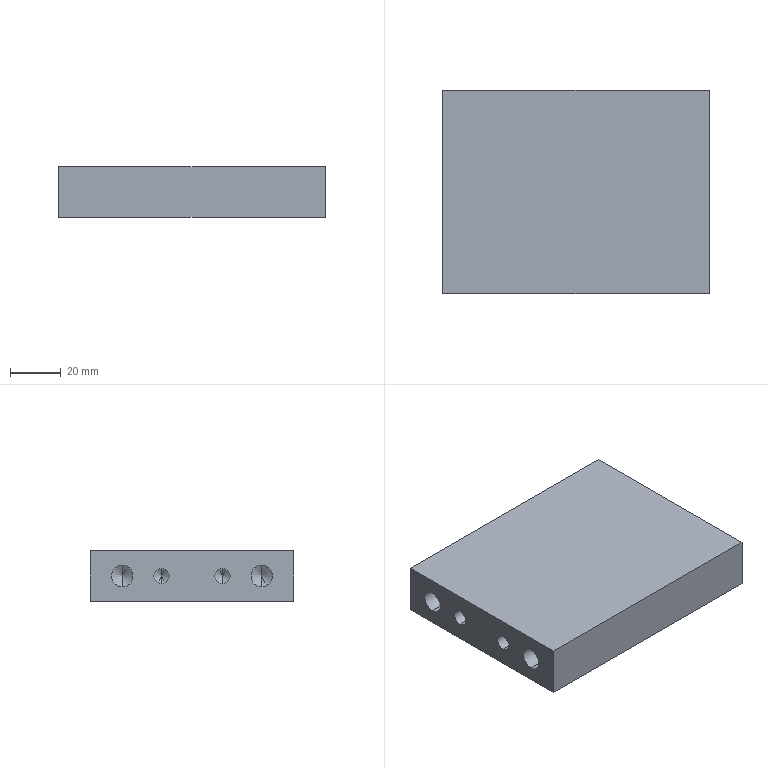Part | STEP file | PN_0028 | 1 solid | 38 faces | box 105 x 80 x 20 mm | volume 160821 mm3 | cylinder 16 | cone 16 | plane 6 | commonest cylinder face diameters 6 x8 8.5 x8